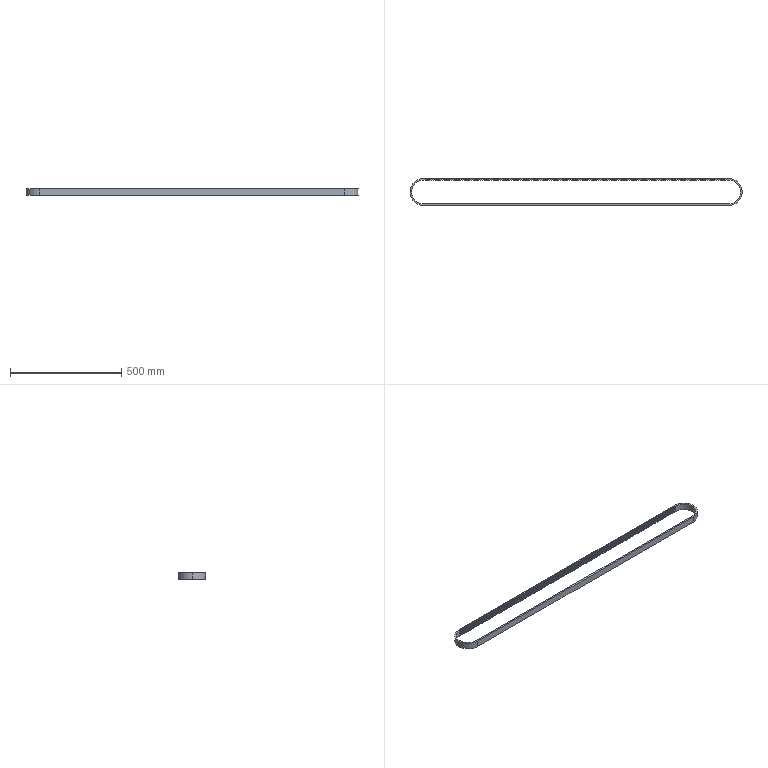Part | SolidWorks | features BaseBody 1 | 1 solid | 556 faces | box 1492 x 121.59 x 30 mm | volume 579141 mm3 | plane 550 | cylinder 6 | commonest cylinder face diameters 107.59 x3 121.59 x3